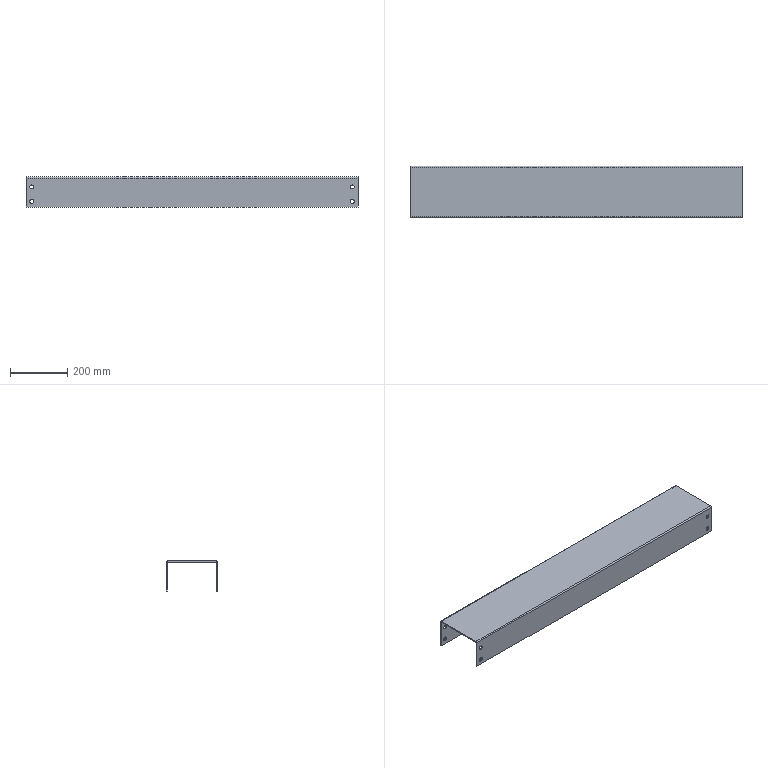Part | SolidWorks | features FlatPattern 1, ICE 1, SMBaseFlange 1, SheetMetal 1 | 1 solid | 38 faces | box 1160 x 180 x 105 mm | volume 1758791 mm3 | cylinder 20 | plane 18 | commonest cylinder face diameters 14 x16 0.4 x2 8.4 x2
STEP:
#1=CARTESIAN_POINT('',(560.,-90.,-92.));
#2=VERTEX_POINT('',#1);
#3=CARTESIAN_POINT('',(560.,-90.,-78.));
#4=VERTEX_POINT('',#3);
#5=CARTESIAN_POINT('',(560.,-90.,-85.));
#6=DIRECTION('',(0.,1.,0.));
#7=DIRECTION('',(0.,0.,1.));
#8=AXIS2_PLACEMENT_3D('',#5,#6,#7);
#9=CIRCLE('',#8,7.);
#10=EDGE_CURVE('',#2,#4,#9,.T.);
#11=ORIENTED_EDGE('',*,*,#10,.F.);
#12=CARTESIAN_POINT('',(560.,-86.,-92.));
#13=VERTEX_POINT('',#12);
#14=CARTESIAN_POINT('',(560.,-324.,-92.));
#15=DIRECTION('',(0.,1.,0.));
#16=VECTOR('',#15,1000.);
#17=LINE('',#14,#16);
#18=EDGE_CURVE('',#2,#13,#17,.T.);
#19=ORIENTED_EDGE('',*,*,#18,.T.);
#20=CARTESIAN_POINT('',(560.,-86.,-78.));
#21=VERTEX_POINT('',#20);
#22=CARTESIAN_POINT('',(560.,-86.,-85.));
#23=DIRECTION('',(0.,1.,0.));
#24=DIRECTION('',(0.,0.,1.));
#25=AXIS2_PLACEMENT_3D('',#22,#23,#24);
#26=CIRCLE('',#25,7.);
#27=EDGE_CURVE('',#13,#21,#26,.T.);
#28=ORIENTED_EDGE('',*,*,#27,.T.);
#29=CARTESIAN_POINT('',(560.,-324.,-78.));
#30=DIRECTION('',(0.,1.,0.));
#31=VECTOR('',#30,1000.);
#32=LINE('',#29,#31);
#33=EDGE_CURVE('',#4,#21,#32,.T.);
#34=ORIENTED_EDGE('',*,*,#33,.F.);
#35=EDGE_LOOP('',(#11,#19,#28,#34));
#36=FACE_OUTER_BOUND('',#35,.T.);
#37=CARTESIAN_POINT('',(560.,-324.,-85.));
#38=DIRECTION('',(0.,1.,0.));
#39=DIRECTION('',(0.,0.,1.));
#40=AXIS2_PLACEMENT_3D('',#37,#38,#39);
#41=CYLINDRICAL_SURFACE('',#40,7.);
#42=ADVANCED_FACE('',(#36),#41,.F.);
#43=CARTESIAN_POINT('',(560.,-90.,-42.));
#44=VERTEX_POINT('',#43);
#45=CARTESIAN_POINT('',(560.,-90.,-28.));
#46=VERTEX_POINT('',#45);
#47=CARTESIAN_POINT('',(560.,-90.,-35.));
#48=DIRECTION('',(0.,1.,0.));
#49=DIRECTION('',(0.,0.,1.));
#50=AXIS2_PLACEMENT_3D('',#47,#48,#49);
#51=CIRCLE('',#50,7.);
#52=EDGE_CURVE('',#44,#46,#51,.T.);
#53=ORIENTED_EDGE('',*,*,#52,.F.);
#54=CARTESIAN_POINT('',(560.,-86.,-42.));
#55=VERTEX_POINT('',#54);
#56=CARTESIAN_POINT('',(560.,-324.,-42.));
#57=DIRECTION('',(0.,1.,0.));
#58=VECTOR('',#57,1000.);
#59=LINE('',#56,#58);
#60=EDGE_CURVE('',#44,#55,#59,.T.);
#61=ORIENTED_EDGE('',*,*,#60,.T.);
#62=CARTESIAN_POINT('',(560.,-86.,-28.));
#63=VERTEX_POINT('',#62);
#64=CARTESIAN_POINT('',(560.,-86.,-35.));
#65=DIRECTION('',(0.,1.,0.));
#66=DIRECTION('',(0.,0.,1.));
#67=AXIS2_PLACEMENT_3D('',#64,#65,#66);
#68=CIRCLE('',#67,7.);
#69=EDGE_CURVE('',#55,#63,#68,.T.);
#70=ORIENTED_EDGE('',*,*,#69,.T.);
#71=CARTESIAN_POINT('',(560.,-324.,-28.));
#72=DIRECTION('',(0.,1.,0.));
#73=VECTOR('',#72,1000.);
#74=LINE('',#71,#73);
#75=EDGE_CURVE('',#46,#63,#74,.T.);
#76=ORIENTED_EDGE('',*,*,#75,.F.);
#77=EDGE_LOOP('',(#53,#61,#70,#76));
#78=FACE_OUTER_BOUND('',#77,.T.);
#79=CARTESIAN_POINT('',(560.,-324.,-35.));
#80=DIRECTION('',(0.,1.,0.));
#81=DIRECTION('',(0.,0.,1.));
#82=AXIS2_PLACEMENT_3D('',#79,#80,#81);
#83=CYLINDRICAL_SURFACE('',#82,7.);
#84=ADVANCED_FACE('',(#78),#83,.F.);
#85=CARTESIAN_POINT('',(-560.,-90.,-42.));
#86=VERTEX_POINT('',#85);
#87=CARTESIAN_POINT('',(-560.,-90.,-28.));
#88=VERTEX_POINT('',#87);
#89=CARTESIAN_POINT('',(-560.,-90.,-35.));
#90=DIRECTION('',(0.,1.,0.));
#91=DIRECTION('',(0.,0.,1.));
#92=AXIS2_PLACEMENT_3D('',#89,#90,#91);
#93=CIRCLE('',#92,7.);
#94=EDGE_CURVE('',#86,#88,#93,.T.);
#95=ORIENTED_EDGE('',*,*,#94,.F.);
#96=CARTESIAN_POINT('',(-560.,-86.,-42.));
#97=VERTEX_POINT('',#96);
#98=CARTESIAN_POINT('',(-560.,-324.,-42.));
#99=DIRECTION('',(0.,1.,0.));
#100=VECTOR('',#99,1000.);
#101=LINE('',#98,#100);
#102=EDGE_CURVE('',#86,#97,#101,.T.);
#103=ORIENTED_EDGE('',*,*,#102,.T.);
#104=CARTESIAN_POINT('',(-560.,-86.,-28.));
#105=VERTEX_POINT('',#104);
#106=CARTESIAN_POINT('',(-560.,-86.,-35.));
#107=DIRECTION('',(0.,1.,0.));
#108=DIRECTION('',(0.,0.,1.));
#109=AXIS2_PLACEMENT_3D('',#106,#107,#108);
#110=CIRCLE('',#109,7.);
#111=EDGE_CURVE('',#97,#105,#110,.T.);
#112=ORIENTED_EDGE('',*,*,#111,.T.);
#113=CARTESIAN_POINT('',(-560.,-324.,-28.));
#114=DIRECTION('',(0.,1.,0.));
#115=VECTOR('',#114,1000.);
#116=LINE('',#113,#115);
#117=EDGE_CURVE('',#88,#105,#116,.T.);
#118=ORIENTED_EDGE('',*,*,#117,.F.);
#119=EDGE_LOOP('',(#95,#103,#112,#118));
#120=FACE_OUTER_BOUND('',#119,.T.);
#121=CARTESIAN_POINT('',(-560.,-324.,-35.));
#122=DIRECTION('',(0.,1.,0.));
#123=DIRECTION('',(0.,0.,1.));
#124=AXIS2_PLACEMENT_3D('',#121,#122,#123);
#125=CYLINDRICAL_SURFACE('',#124,7.);
#126=ADVANCED_FACE('',(#120),#125,.F.);
#127=CARTESIAN_POINT('',(-560.,-90.,-92.));
#128=VERTEX_POINT('',#127);
#129=CARTESIAN_POINT('',(-560.,-90.,-78.));
#130=VERTEX_POINT('',#129);
#131=CARTESIAN_POINT('',(-560.,-90.,-85.));
#132=DIRECTION('',(0.,1.,0.));
#133=DIRECTION('',(0.,0.,1.));
#134=AXIS2_PLACEMENT_3D('',#131,#132,#133);
#135=CIRCLE('',#134,7.);
#136=EDGE_CURVE('',#128,#130,#135,.T.);
#137=ORIENTED_EDGE('',*,*,#136,.F.);
#138=CARTESIAN_POINT('',(-560.,-86.,-92.));
#139=VERTEX_POINT('',#138);
#140=CARTESIAN_POINT('',(-560.,-324.,-92.));
#141=DIRECTION('',(0.,1.,0.));
#142=VECTOR('',#141,1000.);
#143=LINE('',#140,#142);
#144=EDGE_CURVE('',#128,#139,#143,.T.);
#145=ORIENTED_EDGE('',*,*,#144,.T.);
#146=CARTESIAN_POINT('',(-560.,-86.,-78.));
#147=VERTEX_POINT('',#146);
#148=CARTESIAN_POINT('',(-560.,-86.,-85.));
#149=DIRECTION('',(0.,1.,0.));
#150=DIRECTION('',(0.,0.,1.));
#151=AXIS2_PLACEMENT_3D('',#148,#149,#150);
#152=CIRCLE('',#151,7.);
#153=EDGE_CURVE('',#139,#147,#152,.T.);
#154=ORIENTED_EDGE('',*,*,#153,.T.);
#155=CARTESIAN_POINT('',(-560.,-324.,-78.));
#156=DIRECTION('',(0.,1.,0.));
#157=VECTOR('',#156,1000.);
#158=LINE('',#155,#157);
#159=EDGE_CURVE('',#130,#147,#158,.T.);
#160=ORIENTED_EDGE('',*,*,#159,.F.);
#161=EDGE_LOOP('',(#137,#145,#154,#160));
#162=FACE_OUTER_BOUND('',#161,.T.);
#163=CARTESIAN_POINT('',(-560.,-324.,-85.));
#164=DIRECTION('',(0.,1.,0.));
#165=DIRECTION('',(0.,0.,1.));
#166=AXIS2_PLACEMENT_3D('',#163,#164,#165);
#167=CYLINDRICAL_SURFACE('',#166,7.);
#168=ADVANCED_FACE('',(#162),#167,.F.);
#169=CARTESIAN_POINT('',(560.,86.,-78.));
#170=VERTEX_POINT('',#169);
#171=CARTESIAN_POINT('',(560.,86.,-92.));
#172=VERTEX_POINT('',#171);
#173=CARTESIAN_POINT('',(560.,86.,-85.));
#174=DIRECTION('',(0.,-1.,0.));
#175=DIRECTION('',(0.,0.,-1.));
#176=AXIS2_PLACEMENT_3D('',#173,#174,#175);
#177=CIRCLE('',#176,7.);
#178=EDGE_CURVE('',#170,#172,#177,.T.);
#179=ORIENTED_EDGE('',*,*,#178,.T.);
#180=CARTESIAN_POINT('',(560.,90.,-92.));
#181=VERTEX_POINT('',#180);
#182=CARTESIAN_POINT('',(560.,-324.,-92.));
#183=DIRECTION('',(0.,1.,0.));
#184=VECTOR('',#183,1000.);
#185=LINE('',#182,#184);
#186=EDGE_CURVE('',#172,#181,#185,.T.);
#187=ORIENTED_EDGE('',*,*,#186,.T.);
#188=CARTESIAN_POINT('',(560.,90.,-78.));
#189=VERTEX_POINT('',#188);
#190=CARTESIAN_POINT('',(560.,90.,-85.));
#191=DIRECTION('',(0.,1.,0.));
#192=DIRECTION('',(0.,0.,-1.));
#193=AXIS2_PLACEMENT_3D('',#190,#191,#192);
#194=CIRCLE('',#193,7.);
#195=EDGE_CURVE('',#181,#189,#194,.T.);
#196=ORIENTED_EDGE('',*,*,#195,.T.);
#197=CARTESIAN_POINT('',(560.,-324.,-78.));
#198=DIRECTION('',(0.,1.,0.));
#199=VECTOR('',#198,1000.);
#200=LINE('',#197,#199);
#201=EDGE_CURVE('',#170,#189,#200,.T.);
#202=ORIENTED_EDGE('',*,*,#201,.F.);
#203=EDGE_LOOP('',(#179,#187,#196,#202));
#204=FACE_OUTER_BOUND('',#203,.T.);
#205=CARTESIAN_POINT('',(560.,-324.,-85.));
#206=DIRECTION('',(0.,1.,0.));
#207=DIRECTION('',(0.,0.,1.));
#208=AXIS2_PLACEMENT_3D('',#205,#206,#207);
#209=CYLINDRICAL_SURFACE('',#208,7.);
#210=ADVANCED_FACE('',(#204),#209,.F.);
#211=CARTESIAN_POINT('',(560.,86.,-28.));
#212=VERTEX_POINT('',#211);
#213=CARTESIAN_POINT('',(560.,86.,-42.));
#214=VERTEX_POINT('',#213);
#215=CARTESIAN_POINT('',(560.,86.,-35.));
#216=DIRECTION('',(0.,-1.,0.));
#217=DIRECTION('',(0.,0.,-1.));
#218=AXIS2_PLACEMENT_3D('',#215,#216,#217);
#219=CIRCLE('',#218,7.);
#220=EDGE_CURVE('',#212,#214,#219,.T.);
#221=ORIENTED_EDGE('',*,*,#220,.T.);
#222=CARTESIAN_POINT('',(560.,90.,-42.));
#223=VERTEX_POINT('',#222);
#224=CARTESIAN_POINT('',(560.,-324.,-42.));
#225=DIRECTION('',(0.,1.,0.));
#226=VECTOR('',#225,1000.);
#227=LINE('',#224,#226);
#228=EDGE_CURVE('',#214,#223,#227,.T.);
#229=ORIENTED_EDGE('',*,*,#228,.T.);
#230=CARTESIAN_POINT('',(560.,90.,-28.));
#231=VERTEX_POINT('',#230);
#232=CARTESIAN_POINT('',(560.,90.,-35.));
#233=DIRECTION('',(0.,1.,0.));
#234=DIRECTION('',(0.,0.,-1.));
#235=AXIS2_PLACEMENT_3D('',#232,#233,#234);
#236=CIRCLE('',#235,7.);
#237=EDGE_CURVE('',#223,#231,#236,.T.);
#238=ORIENTED_EDGE('',*,*,#237,.T.);
#239=CARTESIAN_POINT('',(560.,-324.,-28.));
#240=DIRECTION('',(0.,1.,0.));
#241=VECTOR('',#240,1000.);
#242=LINE('',#239,#241);
#243=EDGE_CURVE('',#212,#231,#242,.T.);
#244=ORIENTED_EDGE('',*,*,#243,.F.);
#245=EDGE_LOOP('',(#221,#229,#238,#244));
#246=FACE_OUTER_BOUND('',#245,.T.);
#247=CARTESIAN_POINT('',(560.,-324.,-35.));
#248=DIRECTION('',(0.,1.,0.));
#249=DIRECTION('',(0.,0.,1.));
#250=AXIS2_PLACEMENT_3D('',#247,#248,#249);
#251=CYLINDRICAL_SURFACE('',#250,7.);
#252=ADVANCED_FACE('',(#246),#251,.F.);
#253=CARTESIAN_POINT('',(-560.,86.,-28.));
#254=VERTEX_POINT('',#253);
#255=CARTESIAN_POINT('',(-560.,86.,-42.));
#256=VERTEX_POINT('',#255);
#257=CARTESIAN_POINT('',(-560.,86.,-35.));
#258=DIRECTION('',(0.,-1.,0.));
#259=DIRECTION('',(0.,0.,-1.));
#260=AXIS2_PLACEMENT_3D('',#257,#258,#259);
#261=CIRCLE('',#260,7.);
#262=EDGE_CURVE('',#254,#256,#261,.T.);
#263=ORIENTED_EDGE('',*,*,#262,.T.);
#264=CARTESIAN_POINT('',(-560.,90.,-42.));
#265=VERTEX_POINT('',#264);
#266=CARTESIAN_POINT('',(-560.,-324.,-42.));
#267=DIRECTION('',(0.,1.,0.));
#268=VECTOR('',#267,1000.);
#269=LINE('',#266,#268);
#270=EDGE_CURVE('',#256,#265,#269,.T.);
#271=ORIENTED_EDGE('',*,*,#270,.T.);
#272=CARTESIAN_POINT('',(-560.,90.,-28.));
#273=VERTEX_POINT('',#272);
#274=CARTESIAN_POINT('',(-560.,90.,-35.));
#275=DIRECTION('',(0.,1.,0.));
#276=DIRECTION('',(0.,0.,1.));
#277=AXIS2_PLACEMENT_3D('',#274,#275,#276);
#278=CIRCLE('',#277,7.);
#279=EDGE_CURVE('',#265,#273,#278,.T.);
#280=ORIENTED_EDGE('',*,*,#279,.T.);
#281=CARTESIAN_POINT('',(-560.,-324.,-28.));
#282=DIRECTION('',(0.,1.,0.));
#283=VECTOR('',#282,1000.);
#284=LINE('',#281,#283);
#285=EDGE_CURVE('',#254,#273,#284,.T.);
#286=ORIENTED_EDGE('',*,*,#285,.F.);
#287=EDGE_LOOP('',(#263,#271,#280,#286));
#288=FACE_OUTER_BOUND('',#287,.T.);
#289=CARTESIAN_POINT('',(-560.,-324.,-35.));
#290=DIRECTION('',(0.,1.,0.));
#291=DIRECTION('',(0.,0.,1.));
#292=AXIS2_PLACEMENT_3D('',#289,#290,#291);
#293=CYLINDRICAL_SURFACE('',#292,7.);
#294=ADVANCED_FACE('',(#288),#293,.F.);
#295=CARTESIAN_POINT('',(-560.,86.,-78.));
#296=VERTEX_POINT('',#295);
#297=CARTESIAN_POINT('',(-560.,86.,-92.));
#298=VERTEX_POINT('',#297);
#299=CARTESIAN_POINT('',(-560.,86.,-85.));
#300=DIRECTION('',(0.,-1.,0.));
#301=DIRECTION('',(0.,0.,-1.));
#302=AXIS2_PLACEMENT_3D('',#299,#300,#301);
#303=CIRCLE('',#302,7.);
#304=EDGE_CURVE('',#296,#298,#303,.T.);
#305=ORIENTED_EDGE('',*,*,#304,.T.);
#306=CARTESIAN_POINT('',(-560.,90.,-92.));
#307=VERTEX_POINT('',#306);
#308=CARTESIAN_POINT('',(-560.,-324.,-92.));
#309=DIRECTION('',(0.,1.,0.));
#310=VECTOR('',#309,1000.);
#311=LINE('',#308,#310);
#312=EDGE_CURVE('',#298,#307,#311,.T.);
#313=ORIENTED_EDGE('',*,*,#312,.T.);
#314=CARTESIAN_POINT('',(-560.,90.,-78.));
#315=VERTEX_POINT('',#314);
#316=CARTESIAN_POINT('',(-560.,90.,-85.));
#317=DIRECTION('',(0.,1.,0.));
#318=DIRECTION('',(0.,0.,1.));
#319=AXIS2_PLACEMENT_3D('',#316,#317,#318);
#320=CIRCLE('',#319,7.);
#321=EDGE_CURVE('',#307,#315,#320,.T.);
#322=ORIENTED_EDGE('',*,*,#321,.T.);
#323=CARTESIAN_POINT('',(-560.,-324.,-78.));
#324=DIRECTION('',(0.,1.,0.));
#325=VECTOR('',#324,1000.);
#326=LINE('',#323,#325);
#327=EDGE_CURVE('',#296,#315,#326,.T.);
#328=ORIENTED_EDGE('',*,*,#327,.F.);
#329=EDGE_LOOP('',(#305,#313,#322,#328));
#330=FACE_OUTER_BOUND('',#329,.T.);
#331=CARTESIAN_POINT('',(-560.,-324.,-85.));
#332=DIRECTION('',(0.,1.,0.));
#333=DIRECTION('',(0.,0.,1.));
#334=AXIS2_PLACEMENT_3D('',#331,#332,#333);
#335=CYLINDRICAL_SURFACE('',#334,7.);
#336=ADVANCED_FACE('',(#330),#335,.F.);
#337=CARTESIAN_POINT('',(580.,90.,-4.2));
#338=VERTEX_POINT('',#337);
#339=CARTESIAN_POINT('',(580.,86.,-4.2));
#340=VERTEX_POINT('',#339);
#341=CARTESIAN_POINT('',(580.,90.,-4.2));
#342=DIRECTION('',(0.,-1.,0.));
#343=VECTOR('',#342,1000.);
#344=LINE('',#341,#343);
#345=EDGE_CURVE('',#338,#340,#344,.T.);
#346=ORIENTED_EDGE('',*,*,#345,.F.);
#347=CARTESIAN_POINT('',(580.,85.8,0.));
#348=VERTEX_POINT('',#347);
#349=CARTESIAN_POINT('',(580.,85.8,-4.2));
#350=DIRECTION('',(1.,0.,0.));
#351=DIRECTION('',(0.,0.,1.));
#352=AXIS2_PLACEMENT_3D('',#349,#350,#351);
#353=CIRCLE('',#352,4.2);
#354=EDGE_CURVE('',#338,#348,#353,.T.);
#355=ORIENTED_EDGE('',*,*,#354,.T.);
#356=CARTESIAN_POINT('',(580.,85.8,-4.));
#357=VERTEX_POINT('',#356);
#358=CARTESIAN_POINT('',(580.,85.8,-4.));
#359=DIRECTION('',(0.,0.,1.));
#360=VECTOR('',#359,1000.);
#361=LINE('',#358,#360);
#362=EDGE_CURVE('',#357,#348,#361,.T.);
#363=ORIENTED_EDGE('',*,*,#362,.F.);
#364=CARTESIAN_POINT('',(580.,85.8,-4.2));
#365=DIRECTION('',(1.,0.,0.));
#366=DIRECTION('',(0.,0.,-1.));
#367=AXIS2_PLACEMENT_3D('',#364,#365,#366);
#368=CIRCLE('',#367,0.2);
#369=EDGE_CURVE('',#340,#357,#368,.T.);
#370=ORIENTED_EDGE('',*,*,#369,.F.);
#371=EDGE_LOOP('',(#346,#355,#363,#370));
#372=FACE_OUTER_BOUND('',#371,.T.);
#373=CARTESIAN_POINT('',(580.,90.,-4.2));
#374=DIRECTION('',(1.,0.,0.));
#375=DIRECTION('',(0.,0.,-1.));
#376=AXIS2_PLACEMENT_3D('',#373,#374,#375);
#377=PLANE('',#376);
#378=ADVANCED_FACE('',(#372),#377,.T.);
#379=CARTESIAN_POINT('',(580.,90.,-105.));
#380=VERTEX_POINT('',#379);
#381=CARTESIAN_POINT('',(580.,90.,-105.));
#382=DIRECTION('',(0.,0.,1.));
#383=VECTOR('',#382,1000.);
#384=LINE('',#381,#383);
#385=EDGE_CURVE('',#380,#338,#384,.T.);
#386=ORIENTED_EDGE('',*,*,#385,.T.);
#387=ORIENTED_EDGE('',*,*,#345,.T.);
#388=CARTESIAN_POINT('',(580.,86.,-105.));
#389=VERTEX_POINT('',#388);
#390=CARTESIAN_POINT('',(580.,86.,-105.));
#391=DIRECTION('',(0.,0.,1.));
#392=VECTOR('',#391,1000.);
#393=LINE('',#390,#392);
#394=EDGE_CURVE('',#389,#340,#393,.T.);
#395=ORIENTED_EDGE('',*,*,#394,.F.);
#396=CARTESIAN_POINT('',(580.,90.,-105.));
#397=DIRECTION('',(0.,-1.,0.));
#398=VECTOR('',#397,1000.);
#399=LINE('',#396,#398);
#400=EDGE_CURVE('',#380,#389,#399,.T.);
#401=ORIENTED_EDGE('',*,*,#400,.F.);
#402=EDGE_LOOP('',(#386,#387,#395,#401));
#403=FACE_OUTER_BOUND('',#402,.T.);
#404=CARTESIAN_POINT('',(580.,85.8,-4.));
#405=DIRECTION('',(1.,0.,0.));
#406=DIRECTION('',(0.,0.,-1.));
#407=AXIS2_PLACEMENT_3D('',#404,#405,#406);
#408=PLANE('',#407);
#409=ADVANCED_FACE('',(#403),#408,.T.);
#410=CARTESIAN_POINT('',(-580.,85.8,0.));
#411=VERTEX_POINT('',#410);
#412=CARTESIAN_POINT('',(-580.,85.8,-4.));
#413=VERTEX_POINT('',#412);
#414=CARTESIAN_POINT('',(-580.,85.8,0.));
#415=DIRECTION('',(0.,0.,-1.));
#416=VECTOR('',#415,1000.);
#417=LINE('',#414,#416);
#418=EDGE_CURVE('',#411,#413,#417,.T.);
#419=ORIENTED_EDGE('',*,*,#418,.F.);
#420=CARTESIAN_POINT('',(-580.,90.,-4.2));
#421=VERTEX_POINT('',#420);
#422=CARTESIAN_POINT('',(-580.,85.8,-4.2));
#423=DIRECTION('',(1.,0.,0.));
#424=DIRECTION('',(0.,0.,1.));
#425=AXIS2_PLACEMENT_3D('',#422,#423,#424);
#426=CIRCLE('',#425,4.2);
#427=EDGE_CURVE('',#421,#411,#426,.T.);
#428=ORIENTED_EDGE('',*,*,#427,.F.);
#429=CARTESIAN_POINT('',(-580.,86.,-4.2));
#430=VERTEX_POINT('',#429);
#431=CARTESIAN_POINT('',(-580.,86.,-4.2));
#432=DIRECTION('',(0.,1.,0.));
#433=VECTOR('',#432,1000.);
#434=LINE('',#431,#433);
#435=EDGE_CURVE('',#430,#421,#434,.T.);
#436=ORIENTED_EDGE('',*,*,#435,.F.);
#437=CARTESIAN_POINT('',(-580.,85.8,-4.2));
#438=DIRECTION('',(1.,0.,0.));
#439=DIRECTION('',(0.,0.,-1.));
#440=AXIS2_PLACEMENT_3D('',#437,#438,#439);
#441=CIRCLE('',#440,0.2);
#442=EDGE_CURVE('',#430,#413,#441,.T.);
#443=ORIENTED_EDGE('',*,*,#442,.T.);
#444=EDGE_LOOP('',(#419,#428,#436,#443));
#445=FACE_OUTER_BOUND('',#444,.T.);
#446=CARTESIAN_POINT('',(-580.,85.8,0.));
#447=DIRECTION('',(-1.,0.,0.));
#448=DIRECTION('',(0.,0.,1.));
#449=AXIS2_PLACEMENT_3D('',#446,#447,#448);
#450=PLANE('',#449);
#451=ADVANCED_FACE('',(#445),#450,.T.);
#452=CARTESIAN_POINT('',(-580.,-85.8,0.));
#453=VERTEX_POINT('',#452);
#454=CARTESIAN_POINT('',(-580.,90.,0.));
#455=DIRECTION('',(0.,-1.,0.));
#456=VECTOR('',#455,1000.);
#457=LINE('',#454,#456);
#458=EDGE_CURVE('',#411,#453,#457,.T.);
#459=ORIENTED_EDGE('',*,*,#458,.F.);
#460=ORIENTED_EDGE('',*,*,#418,.T.);
#461=CARTESIAN_POINT('',(-580.,-85.8,-4.));
#462=VERTEX_POINT('',#461);
#463=CARTESIAN_POINT('',(-580.,90.,-4.));
#464=DIRECTION('',(0.,-1.,0.));
#465=VECTOR('',#464,1000.);
#466=LINE('',#463,#465);
#467=EDGE_CURVE('',#413,#462,#466,.T.);
#468=ORIENTED_EDGE('',*,*,#467,.T.);
#469=CARTESIAN_POINT('',(-580.,-85.8,-4.));
#470=DIRECTION('',(0.,0.,1.));
#471=VECTOR('',#470,1000.);
#472=LINE('',#469,#471);
#473=EDGE_CURVE('',#462,#453,#472,.T.);
#474=ORIENTED_EDGE('',*,*,#473,.T.);
#475=EDGE_LOOP('',(#459,#460,#468,#474));
#476=FACE_OUTER_BOUND('',#475,.T.);
#477=CARTESIAN_POINT('',(-580.,86.,-4.2));
#478=DIRECTION('',(-1.,0.,0.));
#479=DIRECTION('',(0.,0.,1.));
#480=AXIS2_PLACEMENT_3D('',#477,#478,#479);
#481=PLANE('',#480);
#482=ADVANCED_FACE('',(#476),#481,.T.);
#483=CARTESIAN_POINT('',(580.,-85.8,0.));
#484=VERTEX_POINT('',#483);
#485=CARTESIAN_POINT('',(580.,-85.8,-4.));
#486=VERTEX_POINT('',#485);
#487=CARTESIAN_POINT('',(580.,-85.8,0.));
#488=DIRECTION('',(0.,0.,-1.));
#489=VECTOR('',#488,1000.);
#490=LINE('',#487,#489);
#491=EDGE_CURVE('',#484,#486,#490,.T.);
#492=ORIENTED_EDGE('',*,*,#491,.F.);
#493=CARTESIAN_POINT('',(580.,-90.,-4.2));
#494=VERTEX_POINT('',#493);
#495=CARTESIAN_POINT('',(580.,-85.8,-4.2));
#496=DIRECTION('',(1.,0.,0.));
#497=DIRECTION('',(0.,0.,1.));
#498=AXIS2_PLACEMENT_3D('',#495,#496,#497);
#499=CIRCLE('',#498,4.2);
#500=EDGE_CURVE('',#484,#494,#499,.T.);
#501=ORIENTED_EDGE('',*,*,#500,.T.);
#502=CARTESIAN_POINT('',(580.,-86.,-4.2));
#503=VERTEX_POINT('',#502);
#504=CARTESIAN_POINT('',(580.,-86.,-4.2));
#505=DIRECTION('',(0.,-1.,0.));
#506=VECTOR('',#505,1000.);
#507=LINE('',#504,#506);
#508=EDGE_CURVE('',#503,#494,#507,.T.);
#509=ORIENTED_EDGE('',*,*,#508,.F.);
#510=CARTESIAN_POINT('',(580.,-85.8,-4.2));
#511=DIRECTION('',(1.,0.,0.));
#512=DIRECTION('',(0.,0.,-1.));
#513=AXIS2_PLACEMENT_3D('',#510,#511,#512);
#514=CIRCLE('',#513,0.2);
#515=EDGE_CURVE('',#486,#503,#514,.T.);
#516=ORIENTED_EDGE('',*,*,#515,.F.);
#517=EDGE_LOOP('',(#492,#501,#509,#516));
#518=FACE_OUTER_BOUND('',#517,.T.);
#519=CARTESIAN_POINT('',(580.,-85.8,0.));
#520=DIRECTION('',(1.,0.,0.));
#521=DIRECTION('',(0.,0.,-1.));
#522=AXIS2_PLACEMENT_3D('',#519,#520,#521);
#523=PLANE('',#522);
#524=ADVANCED_FACE('',(#518),#523,.T.);
#525=CARTESIAN_POINT('',(580.,90.,0.));
#526=DIRECTION('',(0.,-1.,0.));
#527=VECTOR('',#526,1000.);
#528=LINE('',#525,#527);
#529=EDGE_CURVE('',#348,#484,#528,.T.);
#530=ORIENTED_EDGE('',*,*,#529,.T.);
#531=ORIENTED_EDGE('',*,*,#491,.T.);
#532=CARTESIAN_POINT('',(580.,90.,-4.));
#533=DIRECTION('',(0.,-1.,0.));
#534=VECTOR('',#533,1000.);
#535=LINE('',#532,#534);
#536=EDGE_CURVE('',#357,#486,#535,.T.);
#537=ORIENTED_EDGE('',*,*,#536,.F.);
#538=ORIENTED_EDGE('',*,*,#362,.T.);
#539=EDGE_LOOP('',(#530,#531,#537,#538));
#540=FACE_OUTER_BOUND('',#539,.T.);
#541=CARTESIAN_POINT('',(580.,-86.,-4.2));
#542=DIRECTION('',(1.,0.,0.));
#543=DIRECTION('',(0.,0.,-1.));
#544=AXIS2_PLACEMENT_3D('',#541,#542,#543);
#545=PLANE('',#544);
#546=ADVANCED_FACE('',(#540),#545,.T.);
#547=CARTESIAN_POINT('',(-580.,-90.,-4.2));
#548=VERTEX_POINT('',#547);
#549=CARTESIAN_POINT('',(-580.,-86.,-4.2));
#550=VERTEX_POINT('',#549);
#551=CARTESIAN_POINT('',(-580.,-90.,-4.2));
#552=DIRECTION('',(0.,1.,0.));
#553=VECTOR('',#552,1000.);
#554=LINE('',#551,#553);
#555=EDGE_CURVE('',#548,#550,#554,.T.);
#556=ORIENTED_EDGE('',*,*,#555,.F.);
#557=CARTESIAN_POINT('',(-580.,-85.8,-4.2));
#558=DIRECTION('',(1.,0.,0.));
#559=DIRECTION('',(0.,0.,1.));
#560=AXIS2_PLACEMENT_3D('',#557,#558,#559);
#561=CIRCLE('',#560,4.2);
#562=EDGE_CURVE('',#453,#548,#561,.T.);
#563=ORIENTED_EDGE('',*,*,#562,.F.);
#564=ORIENTED_EDGE('',*,*,#473,.F.);
#565=CARTESIAN_POINT('',(-580.,-85.8,-4.2));
#566=DIRECTION('',(1.,0.,0.));
#567=DIRECTION('',(0.,0.,-1.));
#568=AXIS2_PLACEMENT_3D('',#565,#566,#567);
#569=CIRCLE('',#568,0.2);
#570=EDGE_CURVE('',#462,#550,#569,.T.);
#571=ORIENTED_EDGE('',*,*,#570,.T.);
#572=EDGE_LOOP('',(#556,#563,#564,#571));
#573=FACE_OUTER_BOUND('',#572,.T.);
#574=CARTESIAN_POINT('',(-580.,-90.,-4.2));
#575=DIRECTION('',(-1.,0.,0.));
#576=DIRECTION('',(0.,0.,1.));
#577=AXIS2_PLACEMENT_3D('',#574,#575,#576);
#578=PLANE('',#577);
#579=ADVANCED_FACE('',(#573),#578,.T.);
#580=CARTESIAN_POINT('',(-580.,-90.,-105.));
#581=VERTEX_POINT('',#580);
#582=CARTESIAN_POINT('',(-580.,-90.,0.));
#583=DIRECTION('',(0.,0.,-1.));
#584=VECTOR('',#583,1000.);
#585=LINE('',#582,#584);
#586=EDGE_CURVE('',#548,#581,#585,.T.);
#587=ORIENTED_EDGE('',*,*,#586,.F.);
#588=ORIENTED_EDGE('',*,*,#555,.T.);
#589=CARTESIAN_POINT('',(-580.,-86.,-105.));
#590=VERTEX_POINT('',#589);
#591=CARTESIAN_POINT('',(-580.,-86.,0.));
#592=DIRECTION('',(0.,0.,-1.));
#593=VECTOR('',#592,1000.);
#594=LINE('',#591,#593);
#595=EDGE_CURVE('',#550,#590,#594,.T.);
#596=ORIENTED_EDGE('',*,*,#595,.T.);
#597=CARTESIAN_POINT('',(-580.,-86.,-105.));
#598=DIRECTION('',(0.,-1.,0.));
#599=VECTOR('',#598,1000.);
#600=LINE('',#597,#599);
#601=EDGE_CURVE('',#590,#581,#600,.T.);
#602=ORIENTED_EDGE('',*,*,#601,.T.);
#603=EDGE_LOOP('',(#587,#588,#596,#602));
#604=FACE_OUTER_BOUND('',#603,.T.);
#605=CARTESIAN_POINT('',(-580.,-85.8,-4.));
#606=DIRECTION('',(-1.,0.,0.));
#607=DIRECTION('',(0.,0.,1.));
#608=AXIS2_PLACEMENT_3D('',#605,#606,#607);
#609=PLANE('',#608);
#610=ADVANCED_FACE('',(#604),#609,.T.);
#611=CARTESIAN_POINT('',(560.,-90.,-85.));
#612=DIRECTION('',(0.,1.,0.));
#613=DIRECTION('',(0.,0.,1.));
#614=AXIS2_PLACEMENT_3D('',#611,#612,#613);
#615=CIRCLE('',#614,7.);
#616=EDGE_CURVE('',#4,#2,#615,.T.);
#617=ORIENTED_EDGE('',*,*,#616,.T.);
#618=ORIENTED_EDGE('',*,*,#10,.T.);
#619=EDGE_LOOP('',(#617,#618));
#620=FACE_BOUND('',#619,.T.);
#621=CARTESIAN_POINT('',(560.,-90.,-35.));
#622=DIRECTION('',(0.,1.,0.));
#623=DIRECTION('',(0.,0.,1.));
#624=AXIS2_PLACEMENT_3D('',#621,#622,#623);
#625=CIRCLE('',#624,7.);
#626=EDGE_CURVE('',#46,#44,#625,.T.);
#627=ORIENTED_EDGE('',*,*,#626,.T.);
#628=ORIENTED_EDGE('',*,*,#52,.T.);
#629=EDGE_LOOP('',(#627,#628));
#630=FACE_BOUND('',#629,.T.);
#631=CARTESIAN_POINT('',(-560.,-90.,-35.));
#632=DIRECTION('',(0.,1.,0.));
#633=DIRECTION('',(0.,0.,1.));
#634=AXIS2_PLACEMENT_3D('',#631,#632,#633);
#635=CIRCLE('',#634,7.);
#636=EDGE_CURVE('',#88,#86,#635,.T.);
#637=ORIENTED_EDGE('',*,*,#636,.T.);
#638=ORIENTED_EDGE('',*,*,#94,.T.);
#639=EDGE_LOOP('',(#637,#638));
#640=FACE_BOUND('',#639,.T.);
#641=CARTESIAN_POINT('',(-560.,-90.,-85.));
#642=DIRECTION('',(0.,1.,0.));
#643=DIRECTION('',(0.,0.,1.));
#644=AXIS2_PLACEMENT_3D('',#641,#642,#643);
#645=CIRCLE('',#644,7.);
#646=EDGE_CURVE('',#130,#128,#645,.T.);
#647=ORIENTED_EDGE('',*,*,#646,.T.);
#648=ORIENTED_EDGE('',*,*,#136,.T.);
#649=EDGE_LOOP('',(#647,#648));
#650=FACE_BOUND('',#649,.T.);
#651=ORIENTED_EDGE('',*,*,#586,.T.);
#652=CARTESIAN_POINT('',(580.,-90.,-105.));
#653=VERTEX_POINT('',#652);
#654=CARTESIAN_POINT('',(580.,-90.,-105.));
#655=DIRECTION('',(-1.,0.,0.));
#656=VECTOR('',#655,1000.);
#657=LINE('',#654,#656);
#658=EDGE_CURVE('',#653,#581,#657,.T.);
#659=ORIENTED_EDGE('',*,*,#658,.F.);
#660=CARTESIAN_POINT('',(580.,-90.,0.));
#661=DIRECTION('',(0.,0.,-1.));
#662=VECTOR('',#661,1000.);
#663=LINE('',#660,#662);
#664=EDGE_CURVE('',#494,#653,#663,.T.);
#665=ORIENTED_EDGE('',*,*,#664,.F.);
#666=CARTESIAN_POINT('',(580.,-90.,-4.2));
#667=DIRECTION('',(-1.,0.,0.));
#668=VECTOR('',#667,1000.);
#669=LINE('',#666,#668);
#670=EDGE_CURVE('',#494,#548,#669,.T.);
#671=ORIENTED_EDGE('',*,*,#670,.T.);
#672=EDGE_LOOP('',(#651,#659,#665,#671));
#673=FACE_OUTER_BOUND('',#672,.T.);
#674=CARTESIAN_POINT('',(580.,-90.,0.));
#675=DIRECTION('',(0.,1.,0.));
#676=DIRECTION('',(0.,0.,1.));
#677=AXIS2_PLACEMENT_3D('',#674,#675,#676);
#678=PLANE('',#677);
#679=ADVANCED_FACE('',(#620,#630,#640,#650,#673),#678,.F.);
#680=ORIENTED_EDGE('',*,*,#601,.F.);
#681=CARTESIAN_POINT('',(580.,-86.,-105.));
#682=VERTEX_POINT('',#681);
#683=CARTESIAN_POINT('',(580.,-86.,-105.));
#684=DIRECTION('',(-1.,0.,0.));
#685=VECTOR('',#684,1000.);
#686=LINE('',#683,#685);
#687=EDGE_CURVE('',#682,#590,#686,.T.);
#688=ORIENTED_EDGE('',*,*,#687,.F.);
#689=CARTESIAN_POINT('',(580.,-86.,-105.));
#690=DIRECTION('',(0.,-1.,0.));
#691=VECTOR('',#690,1000.);
#692=LINE('',#689,#691);
#693=EDGE_CURVE('',#682,#653,#692,.T.);
#694=ORIENTED_EDGE('',*,*,#693,.T.);
#695=ORIENTED_EDGE('',*,*,#658,.T.);
#696=EDGE_LOOP('',(#680,#688,#694,#695));
#697=FACE_OUTER_BOUND('',#696,.T.);
#698=CARTESIAN_POINT('',(580.,-86.,-105.));
#699=DIRECTION('',(0.,0.,-1.));
#700=DIRECTION('',(0.,1.,0.));
#701=AXIS2_PLACEMENT_3D('',#698,#699,#700);
#702=PLANE('',#701);
#703=ADVANCED_FACE('',(#697),#702,.T.);
#704=CARTESIAN_POINT('',(560.,-86.,-85.));
#705=DIRECTION('',(0.,1.,0.));
#706=DIRECTION('',(0.,0.,1.));
#707=AXIS2_PLACEMENT_3D('',#704,#705,#706);
#708=CIRCLE('',#707,7.);
#709=EDGE_CURVE('',#21,#13,#708,.T.);
#710=ORIENTED_EDGE('',*,*,#709,.F.);
#711=ORIENTED_EDGE('',*,*,#27,.F.);
#712=EDGE_LOOP('',(#710,#711));
#713=FACE_BOUND('',#712,.T.);
#714=CARTESIAN_POINT('',(560.,-86.,-35.));
#715=DIRECTION('',(0.,1.,0.));
#716=DIRECTION('',(0.,0.,1.));
#717=AXIS2_PLACEMENT_3D('',#714,#715,#716);
#718=CIRCLE('',#717,7.);
#719=EDGE_CURVE('',#63,#55,#718,.T.);
#720=ORIENTED_EDGE('',*,*,#719,.F.);
#721=ORIENTED_EDGE('',*,*,#69,.F.);
#722=EDGE_LOOP('',(#720,#721));
#723=FACE_BOUND('',#722,.T.);
#724=CARTESIAN_POINT('',(-560.,-86.,-35.));
#725=DIRECTION('',(0.,1.,0.));
#726=DIRECTION('',(0.,0.,1.));
#727=AXIS2_PLACEMENT_3D('',#724,#725,#726);
#728=CIRCLE('',#727,7.);
#729=EDGE_CURVE('',#105,#97,#728,.T.);
#730=ORIENTED_EDGE('',*,*,#729,.F.);
#731=ORIENTED_EDGE('',*,*,#111,.F.);
#732=EDGE_LOOP('',(#730,#731));
#733=FACE_BOUND('',#732,.T.);
#734=CARTESIAN_POINT('',(-560.,-86.,-85.));
#735=DIRECTION('',(0.,1.,0.));
#736=DIRECTION('',(0.,0.,1.));
#737=AXIS2_PLACEMENT_3D('',#734,#735,#736);
#738=CIRCLE('',#737,7.);
#739=EDGE_CURVE('',#147,#139,#738,.T.);
#740=ORIENTED_EDGE('',*,*,#739,.F.);
#741=ORIENTED_EDGE('',*,*,#153,.F.);
#742=EDGE_LOOP('',(#740,#741));
#743=FACE_BOUND('',#742,.T.);
#744=ORIENTED_EDGE('',*,*,#595,.F.);
#745=CARTESIAN_POINT('',(580.,-86.,-4.2));
#746=DIRECTION('',(-1.,0.,0.));
#747=VECTOR('',#746,1000.);
#748=LINE('',#745,#747);
#749=EDGE_CURVE('',#503,#550,#748,.T.);
#750=ORIENTED_EDGE('',*,*,#749,.F.);
#751=CARTESIAN_POINT('',(580.,-86.,0.));
#752=DIRECTION('',(0.,0.,-1.));
#753=VECTOR('',#752,1000.);
#754=LINE('',#751,#753);
#755=EDGE_CURVE('',#503,#682,#754,.T.);
#756=ORIENTED_EDGE('',*,*,#755,.T.);
#757=ORIENTED_EDGE('',*,*,#687,.T.);
#758=EDGE_LOOP('',(#744,#750,#756,#757));
#759=FACE_OUTER_BOUND('',#758,.T.);
#760=CARTESIAN_POINT('',(580.,-86.,0.));
#761=DIRECTION('',(0.,1.,0.));
#762=DIRECTION('',(0.,0.,1.));
#763=AXIS2_PLACEMENT_3D('',#760,#761,#762);
#764=PLANE('',#763);
#765=ADVANCED_FACE('',(#713,#723,#733,#743,#759),#764,.T.);
#766=ORIENTED_EDGE('',*,*,#570,.F.);
#767=CARTESIAN_POINT('',(580.,-85.8,-4.));
#768=DIRECTION('',(-1.,0.,0.));
#769=VECTOR('',#768,1000.);
#770=LINE('',#767,#769);
#771=EDGE_CURVE('',#486,#462,#770,.T.);
#772=ORIENTED_EDGE('',*,*,#771,.F.);
#773=ORIENTED_EDGE('',*,*,#515,.T.);
#774=ORIENTED_EDGE('',*,*,#749,.T.);
#775=EDGE_LOOP('',(#766,#772,#773,#774));
#776=FACE_OUTER_BOUND('',#775,.T.);
#777=CARTESIAN_POINT('',(580.,-85.8,-4.2));
#778=DIRECTION('',(-1.,0.,0.));
#779=DIRECTION('',(0.,0.,1.));
#780=AXIS2_PLACEMENT_3D('',#777,#778,#779);
#781=CYLINDRICAL_SURFACE('',#780,0.2);
#782=ADVANCED_FACE('',(#776),#781,.F.);
#783=ORIENTED_EDGE('',*,*,#467,.F.);
#784=CARTESIAN_POINT('',(580.,85.8,-4.));
#785=DIRECTION('',(-1.,0.,0.));
#786=VECTOR('',#785,1000.);
#787=LINE('',#784,#786);
#788=EDGE_CURVE('',#357,#413,#787,.T.);
#789=ORIENTED_EDGE('',*,*,#788,.F.);
#790=ORIENTED_EDGE('',*,*,#536,.T.);
#791=ORIENTED_EDGE('',*,*,#771,.T.);
#792=EDGE_LOOP('',(#783,#789,#790,#791));
#793=FACE_OUTER_BOUND('',#792,.T.);
#794=CARTESIAN_POINT('',(580.,90.,-4.));
#795=DIRECTION('',(0.,0.,-1.));
#796=DIRECTION('',(0.,1.,0.));
#797=AXIS2_PLACEMENT_3D('',#794,#795,#796);
#798=PLANE('',#797);
#799=ADVANCED_FACE('',(#793),#798,.T.);
#800=ORIENTED_EDGE('',*,*,#442,.F.);
#801=CARTESIAN_POINT('',(580.,86.,-4.2));
#802=DIRECTION('',(-1.,0.,0.));
#803=VECTOR('',#802,1000.);
#804=LINE('',#801,#803);
#805=EDGE_CURVE('',#340,#430,#804,.T.);
#806=ORIENTED_EDGE('',*,*,#805,.F.);
#807=ORIENTED_EDGE('',*,*,#369,.T.);
#808=ORIENTED_EDGE('',*,*,#788,.T.);
#809=EDGE_LOOP('',(#800,#806,#807,#808));
#810=FACE_OUTER_BOUND('',#809,.T.);
#811=CARTESIAN_POINT('',(580.,85.8,-4.2));
#812=DIRECTION('',(-1.,0.,0.));
#813=DIRECTION('',(0.,0.,1.));
#814=AXIS2_PLACEMENT_3D('',#811,#812,#813);
#815=CYLINDRICAL_SURFACE('',#814,0.2);
#816=ADVANCED_FACE('',(#810),#815,.F.);
#817=ORIENTED_EDGE('',*,*,#178,.F.);
#818=CARTESIAN_POINT('',(560.,86.,-85.));
#819=DIRECTION('',(0.,-1.,0.));
#820=DIRECTION('',(0.,0.,-1.));
#821=AXIS2_PLACEMENT_3D('',#818,#819,#820);
#822=CIRCLE('',#821,7.);
#823=EDGE_CURVE('',#172,#170,#822,.T.);
#824=ORIENTED_EDGE('',*,*,#823,.F.);
#825=EDGE_LOOP('',(#817,#824));
#826=FACE_BOUND('',#825,.T.);
#827=ORIENTED_EDGE('',*,*,#220,.F.);
#828=CARTESIAN_POINT('',(560.,86.,-35.));
#829=DIRECTION('',(0.,-1.,0.));
#830=DIRECTION('',(0.,0.,-1.));
#831=AXIS2_PLACEMENT_3D('',#828,#829,#830);
#832=CIRCLE('',#831,7.);
#833=EDGE_CURVE('',#214,#212,#832,.T.);
#834=ORIENTED_EDGE('',*,*,#833,.F.);
#835=EDGE_LOOP('',(#827,#834));
#836=FACE_BOUND('',#835,.T.);
#837=ORIENTED_EDGE('',*,*,#262,.F.);
#838=CARTESIAN_POINT('',(-560.,86.,-35.));
#839=DIRECTION('',(0.,-1.,0.));
#840=DIRECTION('',(0.,0.,-1.));
#841=AXIS2_PLACEMENT_3D('',#838,#839,#840);
#842=CIRCLE('',#841,7.);
#843=EDGE_CURVE('',#256,#254,#842,.T.);
#844=ORIENTED_EDGE('',*,*,#843,.F.);
#845=EDGE_LOOP('',(#837,#844));
#846=FACE_BOUND('',#845,.T.);
#847=ORIENTED_EDGE('',*,*,#304,.F.);
#848=CARTESIAN_POINT('',(-560.,86.,-85.));
#849=DIRECTION('',(0.,-1.,0.));
#850=DIRECTION('',(0.,0.,-1.));
#851=AXIS2_PLACEMENT_3D('',#848,#849,#850);
#852=CIRCLE('',#851,7.);
#853=EDGE_CURVE('',#298,#296,#852,.T.);
#854=ORIENTED_EDGE('',*,*,#853,.F.);
#855=EDGE_LOOP('',(#847,#854));
#856=FACE_BOUND('',#855,.T.);
#857=CARTESIAN_POINT('',(-580.,86.,-105.));
#858=VERTEX_POINT('',#857);
#859=CARTESIAN_POINT('',(-580.,86.,-105.));
#860=DIRECTION('',(0.,0.,1.));
#861=VECTOR('',#860,1000.);
#862=LINE('',#859,#861);
#863=EDGE_CURVE('',#858,#430,#862,.T.);
#864=ORIENTED_EDGE('',*,*,#863,.F.);
#865=CARTESIAN_POINT('',(580.,86.,-105.));
#866=DIRECTION('',(-1.,0.,0.));
#867=VECTOR('',#866,1000.);
#868=LINE('',#865,#867);
#869=EDGE_CURVE('',#389,#858,#868,.T.);
#870=ORIENTED_EDGE('',*,*,#869,.F.);
#871=ORIENTED_EDGE('',*,*,#394,.T.);
#872=ORIENTED_EDGE('',*,*,#805,.T.);
#873=EDGE_LOOP('',(#864,#870,#871,#872));
#874=FACE_OUTER_BOUND('',#873,.T.);
#875=CARTESIAN_POINT('',(580.,86.,-105.));
#876=DIRECTION('',(0.,-1.,0.));
#877=DIRECTION('',(0.,0.,-1.));
#878=AXIS2_PLACEMENT_3D('',#875,#876,#877);
#879=PLANE('',#878);
#880=ADVANCED_FACE('',(#826,#836,#846,#856,#874),#879,.T.);
#881=CARTESIAN_POINT('',(-580.,90.,-105.));
#882=VERTEX_POINT('',#881);
#883=CARTESIAN_POINT('',(-580.,90.,-105.));
#884=DIRECTION('',(0.,-1.,0.));
#885=VECTOR('',#884,1000.);
#886=LINE('',#883,#885);
#887=EDGE_CURVE('',#882,#858,#886,.T.);
#888=ORIENTED_EDGE('',*,*,#887,.F.);
#889=CARTESIAN_POINT('',(580.,90.,-105.));
#890=DIRECTION('',(-1.,0.,0.));
#891=VECTOR('',#890,1000.);
#892=LINE('',#889,#891);
#893=EDGE_CURVE('',#380,#882,#892,.T.);
#894=ORIENTED_EDGE('',*,*,#893,.F.);
#895=ORIENTED_EDGE('',*,*,#400,.T.);
#896=ORIENTED_EDGE('',*,*,#869,.T.);
#897=EDGE_LOOP('',(#888,#894,#895,#896));
#898=FACE_OUTER_BOUND('',#897,.T.);
#899=CARTESIAN_POINT('',(580.,90.,-105.));
#900=DIRECTION('',(0.,0.,-1.));
#901=DIRECTION('',(-1.,0.,0.));
#902=AXIS2_PLACEMENT_3D('',#899,#900,#901);
#903=PLANE('',#902);
#904=ADVANCED_FACE('',(#898),#903,.T.);
#905=CARTESIAN_POINT('',(560.,90.,-85.));
#906=DIRECTION('',(0.,1.,0.));
#907=DIRECTION('',(0.,0.,-1.));
#908=AXIS2_PLACEMENT_3D('',#905,#906,#907);
#909=CIRCLE('',#908,7.);
#910=EDGE_CURVE('',#189,#181,#909,.T.);
#911=ORIENTED_EDGE('',*,*,#910,.F.);
#912=ORIENTED_EDGE('',*,*,#195,.F.);
#913=EDGE_LOOP('',(#911,#912));
#914=FACE_BOUND('',#913,.T.);
#915=CARTESIAN_POINT('',(560.,90.,-35.));
#916=DIRECTION('',(0.,1.,0.));
#917=DIRECTION('',(0.,0.,-1.));
#918=AXIS2_PLACEMENT_3D('',#915,#916,#917);
#919=CIRCLE('',#918,7.);
#920=EDGE_CURVE('',#231,#223,#919,.T.);
#921=ORIENTED_EDGE('',*,*,#920,.F.);
#922=ORIENTED_EDGE('',*,*,#237,.F.);
#923=EDGE_LOOP('',(#921,#922));
#924=FACE_BOUND('',#923,.T.);
#925=CARTESIAN_POINT('',(-560.,90.,-35.));
#926=DIRECTION('',(0.,1.,0.));
#927=DIRECTION('',(0.,0.,1.));
#928=AXIS2_PLACEMENT_3D('',#925,#926,#927);
#929=CIRCLE('',#928,7.);
#930=EDGE_CURVE('',#273,#265,#929,.T.);
#931=ORIENTED_EDGE('',*,*,#930,.F.);
#932=ORIENTED_EDGE('',*,*,#279,.F.);
#933=EDGE_LOOP('',(#931,#932));
#934=FACE_BOUND('',#933,.T.);
#935=CARTESIAN_POINT('',(-560.,90.,-85.));
#936=DIRECTION('',(0.,1.,0.));
#937=DIRECTION('',(0.,0.,1.));
#938=AXIS2_PLACEMENT_3D('',#935,#936,#937);
#939=CIRCLE('',#938,7.);
#940=EDGE_CURVE('',#315,#307,#939,.T.);
#941=ORIENTED_EDGE('',*,*,#940,.F.);
#942=ORIENTED_EDGE('',*,*,#321,.F.);
#943=EDGE_LOOP('',(#941,#942));
#944=FACE_BOUND('',#943,.T.);
#945=CARTESIAN_POINT('',(-580.,90.,-105.));
#946=DIRECTION('',(0.,0.,1.));
#947=VECTOR('',#946,1000.);
#948=LINE('',#945,#947);
#949=EDGE_CURVE('',#882,#421,#948,.T.);
#950=ORIENTED_EDGE('',*,*,#949,.T.);
#951=CARTESIAN_POINT('',(580.,90.,-4.2));
#952=DIRECTION('',(-1.,0.,0.));
#953=VECTOR('',#952,1000.);
#954=LINE('',#951,#953);
#955=EDGE_CURVE('',#338,#421,#954,.T.);
#956=ORIENTED_EDGE('',*,*,#955,.F.);
#957=ORIENTED_EDGE('',*,*,#385,.F.);
#958=ORIENTED_EDGE('',*,*,#893,.T.);
#959=EDGE_LOOP('',(#950,#956,#957,#958));
#960=FACE_OUTER_BOUND('',#959,.T.);
#961=CARTESIAN_POINT('',(580.,90.,-105.));
#962=DIRECTION('',(0.,-1.,0.));
#963=DIRECTION('',(0.,0.,-1.));
#964=AXIS2_PLACEMENT_3D('',#961,#962,#963);
#965=PLANE('',#964);
#966=ADVANCED_FACE('',(#914,#924,#934,#944,#960),#965,.F.);
#967=ORIENTED_EDGE('',*,*,#427,.T.);
#968=CARTESIAN_POINT('',(580.,85.8,0.));
#969=DIRECTION('',(-1.,0.,0.));
#970=VECTOR('',#969,1000.);
#971=LINE('',#968,#970);
#972=EDGE_CURVE('',#348,#411,#971,.T.);
#973=ORIENTED_EDGE('',*,*,#972,.F.);
#974=ORIENTED_EDGE('',*,*,#354,.F.);
#975=ORIENTED_EDGE('',*,*,#955,.T.);
#976=EDGE_LOOP('',(#967,#973,#974,#975));
#977=FACE_OUTER_BOUND('',#976,.T.);
#978=CARTESIAN_POINT('',(580.,85.8,-4.2));
#979=DIRECTION('',(-1.,0.,0.));
#980=DIRECTION('',(0.,0.,1.));
#981=AXIS2_PLACEMENT_3D('',#978,#979,#980);
#982=CYLINDRICAL_SURFACE('',#981,4.2);
#983=ADVANCED_FACE('',(#977),#982,.T.);
#984=ORIENTED_EDGE('',*,*,#458,.T.);
#985=CARTESIAN_POINT('',(580.,-85.8,0.));
#986=DIRECTION('',(-1.,0.,0.));
#987=VECTOR('',#986,1000.);
#988=LINE('',#985,#987);
#989=EDGE_CURVE('',#484,#453,#988,.T.);
#990=ORIENTED_EDGE('',*,*,#989,.F.);
#991=ORIENTED_EDGE('',*,*,#529,.F.);
#992=ORIENTED_EDGE('',*,*,#972,.T.);
#993=EDGE_LOOP('',(#984,#990,#991,#992));
#994=FACE_OUTER_BOUND('',#993,.T.);
#995=CARTESIAN_POINT('',(580.,90.,0.));
#996=DIRECTION('',(0.,0.,-1.));
#997=DIRECTION('',(0.,1.,0.));
#998=AXIS2_PLACEMENT_3D('',#995,#996,#997);
#999=PLANE('',#998);
#1000=ADVANCED_FACE('',(#994),#999,.F.);
#1001=ORIENTED_EDGE('',*,*,#562,.T.);
#1002=ORIENTED_EDGE('',*,*,#670,.F.);
#1003=ORIENTED_EDGE('',*,*,#500,.F.);
#1004=ORIENTED_EDGE('',*,*,#989,.T.);
#1005=EDGE_LOOP('',(#1001,#1002,#1003,#1004));
#1006=FACE_OUTER_BOUND('',#1005,.T.);
#1007=CARTESIAN_POINT('',(580.,-85.8,-4.2));
#1008=DIRECTION('',(-1.,0.,0.));
#1009=DIRECTION('',(0.,0.,1.));
#1010=AXIS2_PLACEMENT_3D('',#1007,#1008,#1009);
#1011=CYLINDRICAL_SURFACE('',#1010,4.2);
#1012=ADVANCED_FACE('',(#1006),#1011,.T.);
#1013=ORIENTED_EDGE('',*,*,#664,.T.);
#1014=ORIENTED_EDGE('',*,*,#693,.F.);
#1015=ORIENTED_EDGE('',*,*,#755,.F.);
#1016=ORIENTED_EDGE('',*,*,#508,.T.);
#1017=EDGE_LOOP('',(#1013,#1014,#1015,#1016));
#1018=FACE_OUTER_BOUND('',#1017,.T.);
#1019=CARTESIAN_POINT('',(580.,-85.8,-4.2));
#1020=DIRECTION('',(1.,0.,0.));
#1021=DIRECTION('',(0.,0.,-1.));
#1022=AXIS2_PLACEMENT_3D('',#1019,#1020,#1021);
#1023=PLANE('',#1022);
#1024=ADVANCED_FACE('',(#1018),#1023,.T.);
#1025=ORIENTED_EDGE('',*,*,#863,.T.);
#1026=ORIENTED_EDGE('',*,*,#435,.T.);
#1027=ORIENTED_EDGE('',*,*,#949,.F.);
#1028=ORIENTED_EDGE('',*,*,#887,.T.);
#1029=EDGE_LOOP('',(#1025,#1026,#1027,#1028));
#1030=FACE_OUTER_BOUND('',#1029,.T.);
#1031=CARTESIAN_POINT('',(-580.,-85.8,-4.2));
#1032=DIRECTION('',(1.,0.,0.));
#1033=DIRECTION('',(0.,0.,-1.));
#1034=AXIS2_PLACEMENT_3D('',#1031,#1032,#1033);
#1035=PLANE('',#1034);
#1036=ADVANCED_FACE('',(#1030),#1035,.F.);
#1037=ORIENTED_EDGE('',*,*,#312,.F.);
#1038=ORIENTED_EDGE('',*,*,#853,.T.);
#1039=ORIENTED_EDGE('',*,*,#327,.T.);
#1040=ORIENTED_EDGE('',*,*,#940,.T.);
#1041=EDGE_LOOP('',(#1037,#1038,#1039,#1040));
#1042=FACE_OUTER_BOUND('',#1041,.T.);
#1043=CARTESIAN_POINT('',(-560.,-324.,-85.));
#1044=DIRECTION('',(0.,1.,0.));
#1045=DIRECTION('',(0.,0.,1.));
#1046=AXIS2_PLACEMENT_3D('',#1043,#1044,#1045);
#1047=CYLINDRICAL_SURFACE('',#1046,7.);
#1048=ADVANCED_FACE('',(#1042),#1047,.F.);
#1049=ORIENTED_EDGE('',*,*,#270,.F.);
#1050=ORIENTED_EDGE('',*,*,#843,.T.);
#1051=ORIENTED_EDGE('',*,*,#285,.T.);
#1052=ORIENTED_EDGE('',*,*,#930,.T.);
#1053=EDGE_LOOP('',(#1049,#1050,#1051,#1052));
#1054=FACE_OUTER_BOUND('',#1053,.T.);
#1055=CARTESIAN_POINT('',(-560.,-324.,-35.));
#1056=DIRECTION('',(0.,1.,0.));
#1057=DIRECTION('',(0.,0.,1.));
#1058=AXIS2_PLACEMENT_3D('',#1055,#1056,#1057);
#1059=CYLINDRICAL_SURFACE('',#1058,7.);
#1060=ADVANCED_FACE('',(#1054),#1059,.F.);
#1061=ORIENTED_EDGE('',*,*,#228,.F.);
#1062=ORIENTED_EDGE('',*,*,#833,.T.);
#1063=ORIENTED_EDGE('',*,*,#243,.T.);
#1064=ORIENTED_EDGE('',*,*,#920,.T.);
#1065=EDGE_LOOP('',(#1061,#1062,#1063,#1064));
#1066=FACE_OUTER_BOUND('',#1065,.T.);
#1067=CARTESIAN_POINT('',(560.,-324.,-35.));
#1068=DIRECTION('',(0.,1.,0.));
#1069=DIRECTION('',(0.,0.,1.));
#1070=AXIS2_PLACEMENT_3D('',#1067,#1068,#1069);
#1071=CYLINDRICAL_SURFACE('',#1070,7.);
#1072=ADVANCED_FACE('',(#1066),#1071,.F.);
#1073=ORIENTED_EDGE('',*,*,#186,.F.);
#1074=ORIENTED_EDGE('',*,*,#823,.T.);
#1075=ORIENTED_EDGE('',*,*,#201,.T.);
#1076=ORIENTED_EDGE('',*,*,#910,.T.);
#1077=EDGE_LOOP('',(#1073,#1074,#1075,#1076));
#1078=FACE_OUTER_BOUND('',#1077,.T.);
#1079=CARTESIAN_POINT('',(560.,-324.,-85.));
#1080=DIRECTION('',(0.,1.,0.));
#1081=DIRECTION('',(0.,0.,1.));
#1082=AXIS2_PLACEMENT_3D('',#1079,#1080,#1081);
#1083=CYLINDRICAL_SURFACE('',#1082,7.);
#1084=ADVANCED_FACE('',(#1078),#1083,.F.);
#1085=ORIENTED_EDGE('',*,*,#144,.F.);
#1086=ORIENTED_EDGE('',*,*,#646,.F.);
#1087=ORIENTED_EDGE('',*,*,#159,.T.);
#1088=ORIENTED_EDGE('',*,*,#739,.T.);
#1089=EDGE_LOOP('',(#1085,#1086,#1087,#1088));
#1090=FACE_OUTER_BOUND('',#1089,.T.);
#1091=CARTESIAN_POINT('',(-560.,-324.,-85.));
#1092=DIRECTION('',(0.,1.,0.));
#1093=DIRECTION('',(0.,0.,1.));
#1094=AXIS2_PLACEMENT_3D('',#1091,#1092,#1093);
#1095=CYLINDRICAL_SURFACE('',#1094,7.);
#1096=ADVANCED_FACE('',(#1090),#1095,.F.);
#1097=ORIENTED_EDGE('',*,*,#102,.F.);
#1098=ORIENTED_EDGE('',*,*,#636,.F.);
#1099=ORIENTED_EDGE('',*,*,#117,.T.);
#1100=ORIENTED_EDGE('',*,*,#729,.T.);
#1101=EDGE_LOOP('',(#1097,#1098,#1099,#1100));
#1102=FACE_OUTER_BOUND('',#1101,.T.);
#1103=CARTESIAN_POINT('',(-560.,-324.,-35.));
#1104=DIRECTION('',(0.,1.,0.));
#1105=DIRECTION('',(0.,0.,1.));
#1106=AXIS2_PLACEMENT_3D('',#1103,#1104,#1105);
#1107=CYLINDRICAL_SURFACE('',#1106,7.);
#1108=ADVANCED_FACE('',(#1102),#1107,.F.);
#1109=ORIENTED_EDGE('',*,*,#60,.F.);
#1110=ORIENTED_EDGE('',*,*,#626,.F.);
#1111=ORIENTED_EDGE('',*,*,#75,.T.);
#1112=ORIENTED_EDGE('',*,*,#719,.T.);
#1113=EDGE_LOOP('',(#1109,#1110,#1111,#1112));
#1114=FACE_OUTER_BOUND('',#1113,.T.);
#1115=CARTESIAN_POINT('',(560.,-324.,-35.));
#1116=DIRECTION('',(0.,1.,0.));
#1117=DIRECTION('',(0.,0.,1.));
#1118=AXIS2_PLACEMENT_3D('',#1115,#1116,#1117);
#1119=CYLINDRICAL_SURFACE('',#1118,7.);
#1120=ADVANCED_FACE('',(#1114),#1119,.F.);
#1121=ORIENTED_EDGE('',*,*,#18,.F.);
#1122=ORIENTED_EDGE('',*,*,#616,.F.);
#1123=ORIENTED_EDGE('',*,*,#33,.T.);
#1124=ORIENTED_EDGE('',*,*,#709,.T.);
#1125=EDGE_LOOP('',(#1121,#1122,#1123,#1124));
#1126=FACE_OUTER_BOUND('',#1125,.T.);
#1127=CARTESIAN_POINT('',(560.,-324.,-85.));
#1128=DIRECTION('',(0.,1.,0.));
#1129=DIRECTION('',(0.,0.,1.));
#1130=AXIS2_PLACEMENT_3D('',#1127,#1128,#1129);
#1131=CYLINDRICAL_SURFACE('',#1130,7.);
#1132=ADVANCED_FACE('',(#1126),#1131,.F.);
#1133=CLOSED_SHELL('',(#42,#84,#126,#168,#210,#252,#294,#336,#378,#409,#451,#482,#524,#546,#579,#610,#679,#703,#765,#782,#799,#816,#880,#904,#966,#983,#1000,#1012,#1024,#1036,#1048,#1060,#1072,#1084,#1096,#1108,#1120,#1132));
#1134=MANIFOLD_SOLID_BREP('',#1133);
#1135=CARTESIAN_POINT('',(0.,0.,0.));
#1136=DIRECTION('',(0.,0.,1.));
#1137=DIRECTION('',(1.,0.,0.));
#1138=AXIS2_PLACEMENT_3D('',#1135,#1136,#1137);
#1139=(LENGTH_UNIT()NAMED_UNIT(*)SI_UNIT(.MILLI.,.METRE.));
#1140=UNCERTAINTY_MEASURE_WITH_UNIT(LENGTH_MEASURE(0.00001),#1139,'','');
#1141=(NAMED_UNIT(*)PLANE_ANGLE_UNIT()SI_UNIT($,.RADIAN.));
#1142=(NAMED_UNIT(*)SI_UNIT($,.STERADIAN.)SOLID_ANGLE_UNIT());
#1143=(GEOMETRIC_REPRESENTATION_CONTEXT(3)GLOBAL_UNCERTAINTY_ASSIGNED_CONTEXT((#1140))GLOBAL_UNIT_ASSIGNED_CONTEXT((#1139,#1141,#1142))REPRESENTATION_CONTEXT('',''));
#1144=ADVANCED_BREP_SHAPE_REPRESENTATION('',(#1134,#1138),#1143);